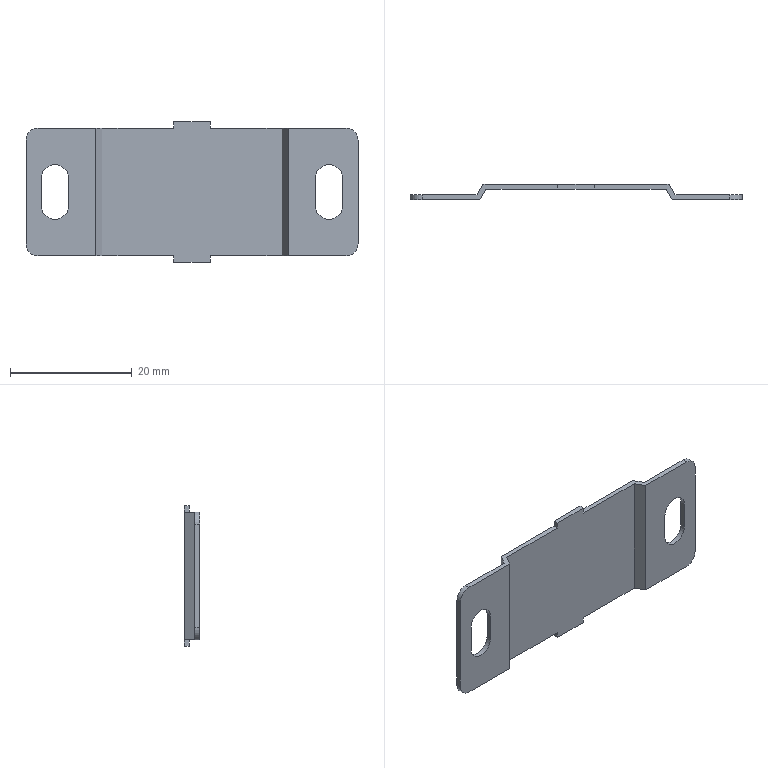Part | STEP file | Second C-100-B-2 Bracket Part | 1 solid | 34 faces | box 54.5 x 2.5 x 23 mm | volume 897.584 mm3 | plane 26 | cylinder 8 | commonest cylinder face diameters 4 x4 4.5 x4
STEP:
#1=CARTESIAN_POINT('',(3.,2.5,-11.5));
#2=VERTEX_POINT('',#1);
#3=CARTESIAN_POINT('',(3.,2.5,-10.5));
#4=VERTEX_POINT('',#3);
#5=CARTESIAN_POINT('',(3.,2.5,10.5));
#6=DIRECTION('',(0.,0.,1.));
#7=VECTOR('',#6,1000.);
#8=LINE('',#5,#7);
#9=EDGE_CURVE('',#2,#4,#8,.T.);
#10=ORIENTED_EDGE('',*,*,#9,.F.);
#11=CARTESIAN_POINT('',(-3.,2.5,-11.5));
#12=VERTEX_POINT('',#11);
#13=CARTESIAN_POINT('',(-15.269,2.5,-11.5));
#14=DIRECTION('',(1.,0.,0.));
#15=VECTOR('',#14,1000.);
#16=LINE('',#13,#15);
#17=EDGE_CURVE('',#12,#2,#16,.T.);
#18=ORIENTED_EDGE('',*,*,#17,.F.);
#19=CARTESIAN_POINT('',(-3.,2.5,-10.5));
#20=VERTEX_POINT('',#19);
#21=CARTESIAN_POINT('',(-3.,2.5,10.5));
#22=DIRECTION('',(0.,0.,-1.));
#23=VECTOR('',#22,1000.);
#24=LINE('',#21,#23);
#25=EDGE_CURVE('',#20,#12,#24,.T.);
#26=ORIENTED_EDGE('',*,*,#25,.F.);
#27=CARTESIAN_POINT('',(-15.269,2.5,-10.5));
#28=VERTEX_POINT('',#27);
#29=CARTESIAN_POINT('',(-15.269,2.5,-10.5));
#30=DIRECTION('',(1.,0.,0.));
#31=VECTOR('',#30,1000.);
#32=LINE('',#29,#31);
#33=EDGE_CURVE('',#28,#20,#32,.T.);
#34=ORIENTED_EDGE('',*,*,#33,.F.);
#35=CARTESIAN_POINT('',(-15.269,2.5,10.5));
#36=VERTEX_POINT('',#35);
#37=CARTESIAN_POINT('',(-15.269,2.5,10.5));
#38=DIRECTION('',(0.,0.,-1.));
#39=VECTOR('',#38,1000.);
#40=LINE('',#37,#39);
#41=EDGE_CURVE('',#36,#28,#40,.T.);
#42=ORIENTED_EDGE('',*,*,#41,.F.);
#43=CARTESIAN_POINT('',(-3.,2.5,10.5));
#44=VERTEX_POINT('',#43);
#45=CARTESIAN_POINT('',(-15.269,2.5,10.5));
#46=DIRECTION('',(-1.,0.,0.));
#47=VECTOR('',#46,1000.);
#48=LINE('',#45,#47);
#49=EDGE_CURVE('',#44,#36,#48,.T.);
#50=ORIENTED_EDGE('',*,*,#49,.F.);
#51=CARTESIAN_POINT('',(-3.,2.5,11.5));
#52=VERTEX_POINT('',#51);
#53=CARTESIAN_POINT('',(-3.,2.5,10.5));
#54=DIRECTION('',(0.,0.,-1.));
#55=VECTOR('',#54,1000.);
#56=LINE('',#53,#55);
#57=EDGE_CURVE('',#52,#44,#56,.T.);
#58=ORIENTED_EDGE('',*,*,#57,.F.);
#59=CARTESIAN_POINT('',(3.,2.5,11.5));
#60=VERTEX_POINT('',#59);
#61=CARTESIAN_POINT('',(-15.269,2.5,11.5));
#62=DIRECTION('',(-1.,0.,0.));
#63=VECTOR('',#62,1000.);
#64=LINE('',#61,#63);
#65=EDGE_CURVE('',#60,#52,#64,.T.);
#66=ORIENTED_EDGE('',*,*,#65,.F.);
#67=CARTESIAN_POINT('',(3.,2.5,10.5));
#68=VERTEX_POINT('',#67);
#69=CARTESIAN_POINT('',(3.,2.5,10.5));
#70=DIRECTION('',(0.,0.,1.));
#71=VECTOR('',#70,1000.);
#72=LINE('',#69,#71);
#73=EDGE_CURVE('',#68,#60,#72,.T.);
#74=ORIENTED_EDGE('',*,*,#73,.F.);
#75=CARTESIAN_POINT('',(15.269,2.5,10.5));
#76=VERTEX_POINT('',#75);
#77=CARTESIAN_POINT('',(-15.269,2.5,10.5));
#78=DIRECTION('',(-1.,0.,0.));
#79=VECTOR('',#78,1000.);
#80=LINE('',#77,#79);
#81=EDGE_CURVE('',#76,#68,#80,.T.);
#82=ORIENTED_EDGE('',*,*,#81,.F.);
#83=CARTESIAN_POINT('',(15.269,2.5,-10.5));
#84=VERTEX_POINT('',#83);
#85=CARTESIAN_POINT('',(15.269,2.5,10.5));
#86=DIRECTION('',(0.,0.,1.));
#87=VECTOR('',#86,1000.);
#88=LINE('',#85,#87);
#89=EDGE_CURVE('',#84,#76,#88,.T.);
#90=ORIENTED_EDGE('',*,*,#89,.F.);
#91=CARTESIAN_POINT('',(-15.269,2.5,-10.5));
#92=DIRECTION('',(1.,0.,0.));
#93=VECTOR('',#92,1000.);
#94=LINE('',#91,#93);
#95=EDGE_CURVE('',#4,#84,#94,.T.);
#96=ORIENTED_EDGE('',*,*,#95,.F.);
#97=EDGE_LOOP('',(#10,#18,#26,#34,#42,#50,#58,#66,#74,#82,#90,#96));
#98=FACE_OUTER_BOUND('',#97,.T.);
#99=CARTESIAN_POINT('',(-15.269,2.5,10.5));
#100=DIRECTION('',(0.,-1.,0.));
#101=DIRECTION('',(1.,0.,0.));
#102=AXIS2_PLACEMENT_3D('',#99,#100,#101);
#103=PLANE('',#102);
#104=ADVANCED_FACE('',(#98),#103,.F.);
#105=CARTESIAN_POINT('',(3.,1.7,-10.5));
#106=VERTEX_POINT('',#105);
#107=CARTESIAN_POINT('',(3.,2.5,-10.5));
#108=DIRECTION('',(0.,-1.,0.));
#109=VECTOR('',#108,1000.);
#110=LINE('',#107,#109);
#111=EDGE_CURVE('',#4,#106,#110,.T.);
#112=ORIENTED_EDGE('',*,*,#111,.F.);
#113=ORIENTED_EDGE('',*,*,#95,.T.);
#114=CARTESIAN_POINT('',(16.25,0.8,-10.5));
#115=VERTEX_POINT('',#114);
#116=CARTESIAN_POINT('',(16.25,0.8,-10.5));
#117=DIRECTION('',(-0.5,0.866,0.));
#118=VECTOR('',#117,1000.);
#119=LINE('',#116,#118);
#120=EDGE_CURVE('',#115,#84,#119,.T.);
#121=ORIENTED_EDGE('',*,*,#120,.F.);
#122=CARTESIAN_POINT('',(25.25,0.8,-10.5));
#123=VERTEX_POINT('',#122);
#124=CARTESIAN_POINT('',(-27.25,0.8,-10.5));
#125=DIRECTION('',(-1.,0.,0.));
#126=VECTOR('',#125,1000.);
#127=LINE('',#124,#126);
#128=EDGE_CURVE('',#123,#115,#127,.T.);
#129=ORIENTED_EDGE('',*,*,#128,.F.);
#130=CARTESIAN_POINT('',(25.25,0.,-10.5));
#131=VERTEX_POINT('',#130);
#132=CARTESIAN_POINT('',(25.25,0.,-10.5));
#133=DIRECTION('',(0.,1.,0.));
#134=VECTOR('',#133,1000.);
#135=LINE('',#132,#134);
#136=EDGE_CURVE('',#131,#123,#135,.T.);
#137=ORIENTED_EDGE('',*,*,#136,.F.);
#138=CARTESIAN_POINT('',(15.788,0.,-10.5));
#139=VERTEX_POINT('',#138);
#140=CARTESIAN_POINT('',(-27.25,0.,-10.5));
#141=DIRECTION('',(1.,0.,0.));
#142=VECTOR('',#141,1000.);
#143=LINE('',#140,#142);
#144=EDGE_CURVE('',#139,#131,#143,.T.);
#145=ORIENTED_EDGE('',*,*,#144,.F.);
#146=CARTESIAN_POINT('',(14.807,1.7,-10.5));
#147=VERTEX_POINT('',#146);
#148=CARTESIAN_POINT('',(14.807,1.7,-10.5));
#149=DIRECTION('',(0.5,-0.866,0.));
#150=VECTOR('',#149,1000.);
#151=LINE('',#148,#150);
#152=EDGE_CURVE('',#147,#139,#151,.T.);
#153=ORIENTED_EDGE('',*,*,#152,.F.);
#154=CARTESIAN_POINT('',(-27.25,1.7,-10.5));
#155=DIRECTION('',(1.,0.,0.));
#156=VECTOR('',#155,1000.);
#157=LINE('',#154,#156);
#158=EDGE_CURVE('',#106,#147,#157,.T.);
#159=ORIENTED_EDGE('',*,*,#158,.F.);
#160=EDGE_LOOP('',(#112,#113,#121,#129,#137,#145,#153,#159));
#161=FACE_OUTER_BOUND('',#160,.T.);
#162=CARTESIAN_POINT('',(-27.25,2.5,-10.5));
#163=DIRECTION('',(0.,0.,1.));
#164=DIRECTION('',(1.,0.,0.));
#165=AXIS2_PLACEMENT_3D('',#162,#163,#164);
#166=PLANE('',#165);
#167=ADVANCED_FACE('',(#161),#166,.F.);
#168=CARTESIAN_POINT('',(3.,1.7,-11.5));
#169=VERTEX_POINT('',#168);
#170=CARTESIAN_POINT('',(3.,1.7,-11.5));
#171=DIRECTION('',(0.,1.,0.));
#172=VECTOR('',#171,1000.);
#173=LINE('',#170,#172);
#174=EDGE_CURVE('',#169,#2,#173,.T.);
#175=ORIENTED_EDGE('',*,*,#174,.T.);
#176=ORIENTED_EDGE('',*,*,#9,.T.);
#177=ORIENTED_EDGE('',*,*,#111,.T.);
#178=CARTESIAN_POINT('',(3.,1.7,-11.5));
#179=DIRECTION('',(0.,0.,-1.));
#180=VECTOR('',#179,1000.);
#181=LINE('',#178,#180);
#182=EDGE_CURVE('',#106,#169,#181,.T.);
#183=ORIENTED_EDGE('',*,*,#182,.T.);
#184=EDGE_LOOP('',(#175,#176,#177,#183));
#185=FACE_OUTER_BOUND('',#184,.T.);
#186=CARTESIAN_POINT('',(3.,1.7,-11.5));
#187=DIRECTION('',(1.,0.,0.));
#188=DIRECTION('',(0.,1.,0.));
#189=AXIS2_PLACEMENT_3D('',#186,#187,#188);
#190=PLANE('',#189);
#191=ADVANCED_FACE('',(#185),#190,.T.);
#192=CARTESIAN_POINT('',(-3.,1.7,-11.5));
#193=VERTEX_POINT('',#192);
#194=CARTESIAN_POINT('',(-3.,1.7,-11.5));
#195=DIRECTION('',(-1.,0.,0.));
#196=VECTOR('',#195,1000.);
#197=LINE('',#194,#196);
#198=EDGE_CURVE('',#169,#193,#197,.T.);
#199=ORIENTED_EDGE('',*,*,#198,.T.);
#200=CARTESIAN_POINT('',(-3.,1.7,-11.5));
#201=DIRECTION('',(0.,1.,0.));
#202=VECTOR('',#201,1000.);
#203=LINE('',#200,#202);
#204=EDGE_CURVE('',#193,#12,#203,.T.);
#205=ORIENTED_EDGE('',*,*,#204,.T.);
#206=ORIENTED_EDGE('',*,*,#17,.T.);
#207=ORIENTED_EDGE('',*,*,#174,.F.);
#208=EDGE_LOOP('',(#199,#205,#206,#207));
#209=FACE_OUTER_BOUND('',#208,.T.);
#210=CARTESIAN_POINT('',(-3.,1.7,-11.5));
#211=DIRECTION('',(0.,0.,-1.));
#212=DIRECTION('',(-1.,0.,0.));
#213=AXIS2_PLACEMENT_3D('',#210,#211,#212);
#214=PLANE('',#213);
#215=ADVANCED_FACE('',(#209),#214,.T.);
#216=ORIENTED_EDGE('',*,*,#204,.F.);
#217=CARTESIAN_POINT('',(-3.,1.7,-10.5));
#218=VERTEX_POINT('',#217);
#219=CARTESIAN_POINT('',(-3.,1.7,11.5));
#220=DIRECTION('',(0.,0.,1.));
#221=VECTOR('',#220,1000.);
#222=LINE('',#219,#221);
#223=EDGE_CURVE('',#193,#218,#222,.T.);
#224=ORIENTED_EDGE('',*,*,#223,.T.);
#225=CARTESIAN_POINT('',(-3.,1.7,-10.5));
#226=DIRECTION('',(0.,1.,0.));
#227=VECTOR('',#226,1000.);
#228=LINE('',#225,#227);
#229=EDGE_CURVE('',#218,#20,#228,.T.);
#230=ORIENTED_EDGE('',*,*,#229,.T.);
#231=ORIENTED_EDGE('',*,*,#25,.T.);
#232=EDGE_LOOP('',(#216,#224,#230,#231));
#233=FACE_OUTER_BOUND('',#232,.T.);
#234=CARTESIAN_POINT('',(-3.,1.7,11.5));
#235=DIRECTION('',(-1.,0.,0.));
#236=DIRECTION('',(0.,0.,1.));
#237=AXIS2_PLACEMENT_3D('',#234,#235,#236);
#238=PLANE('',#237);
#239=ADVANCED_FACE('',(#233),#238,.T.);
#240=ORIENTED_EDGE('',*,*,#229,.F.);
#241=CARTESIAN_POINT('',(-14.807,1.7,-10.5));
#242=VERTEX_POINT('',#241);
#243=CARTESIAN_POINT('',(-27.25,1.7,-10.5));
#244=DIRECTION('',(1.,0.,0.));
#245=VECTOR('',#244,1000.);
#246=LINE('',#243,#245);
#247=EDGE_CURVE('',#242,#218,#246,.T.);
#248=ORIENTED_EDGE('',*,*,#247,.F.);
#249=CARTESIAN_POINT('',(-15.788,0.,-10.5));
#250=VERTEX_POINT('',#249);
#251=CARTESIAN_POINT('',(-15.788,0.,-10.5));
#252=DIRECTION('',(0.5,0.866,0.));
#253=VECTOR('',#252,1000.);
#254=LINE('',#251,#253);
#255=EDGE_CURVE('',#250,#242,#254,.T.);
#256=ORIENTED_EDGE('',*,*,#255,.F.);
#257=CARTESIAN_POINT('',(-25.25,0.,-10.5));
#258=VERTEX_POINT('',#257);
#259=CARTESIAN_POINT('',(-27.25,0.,-10.5));
#260=DIRECTION('',(1.,0.,0.));
#261=VECTOR('',#260,1000.);
#262=LINE('',#259,#261);
#263=EDGE_CURVE('',#258,#250,#262,.T.);
#264=ORIENTED_EDGE('',*,*,#263,.F.);
#265=CARTESIAN_POINT('',(-25.25,0.8,-10.5));
#266=VERTEX_POINT('',#265);
#267=CARTESIAN_POINT('',(-25.25,0.8,-10.5));
#268=DIRECTION('',(0.,-1.,0.));
#269=VECTOR('',#268,1000.);
#270=LINE('',#267,#269);
#271=EDGE_CURVE('',#266,#258,#270,.T.);
#272=ORIENTED_EDGE('',*,*,#271,.F.);
#273=CARTESIAN_POINT('',(-16.25,0.8,-10.5));
#274=VERTEX_POINT('',#273);
#275=CARTESIAN_POINT('',(-27.25,0.8,-10.5));
#276=DIRECTION('',(-1.,0.,0.));
#277=VECTOR('',#276,1000.);
#278=LINE('',#275,#277);
#279=EDGE_CURVE('',#274,#266,#278,.T.);
#280=ORIENTED_EDGE('',*,*,#279,.F.);
#281=CARTESIAN_POINT('',(-15.269,2.5,-10.5));
#282=DIRECTION('',(-0.5,-0.866,0.));
#283=VECTOR('',#282,1000.);
#284=LINE('',#281,#283);
#285=EDGE_CURVE('',#28,#274,#284,.T.);
#286=ORIENTED_EDGE('',*,*,#285,.F.);
#287=ORIENTED_EDGE('',*,*,#33,.T.);
#288=EDGE_LOOP('',(#240,#248,#256,#264,#272,#280,#286,#287));
#289=FACE_OUTER_BOUND('',#288,.T.);
#290=CARTESIAN_POINT('',(-27.25,2.5,-10.5));
#291=DIRECTION('',(0.,0.,1.));
#292=DIRECTION('',(1.,0.,0.));
#293=AXIS2_PLACEMENT_3D('',#290,#291,#292);
#294=PLANE('',#293);
#295=ADVANCED_FACE('',(#289),#294,.F.);
#296=ORIENTED_EDGE('',*,*,#285,.T.);
#297=CARTESIAN_POINT('',(-16.25,0.8,10.5));
#298=VERTEX_POINT('',#297);
#299=CARTESIAN_POINT('',(-16.25,0.8,10.5));
#300=DIRECTION('',(0.,0.,-1.));
#301=VECTOR('',#300,1000.);
#302=LINE('',#299,#301);
#303=EDGE_CURVE('',#298,#274,#302,.T.);
#304=ORIENTED_EDGE('',*,*,#303,.F.);
#305=CARTESIAN_POINT('',(-16.25,0.8,10.5));
#306=DIRECTION('',(-0.5,-0.866,0.));
#307=VECTOR('',#306,1000.);
#308=LINE('',#305,#307);
#309=EDGE_CURVE('',#36,#298,#308,.T.);
#310=ORIENTED_EDGE('',*,*,#309,.F.);
#311=ORIENTED_EDGE('',*,*,#41,.T.);
#312=EDGE_LOOP('',(#296,#304,#310,#311));
#313=FACE_OUTER_BOUND('',#312,.T.);
#314=CARTESIAN_POINT('',(-16.25,0.8,10.5));
#315=DIRECTION('',(0.866,-0.5,0.));
#316=DIRECTION('',(0.5,0.866,0.));
#317=AXIS2_PLACEMENT_3D('',#314,#315,#316);
#318=PLANE('',#317);
#319=ADVANCED_FACE('',(#313),#318,.F.);
#320=CARTESIAN_POINT('',(-15.788,0.,10.5));
#321=VERTEX_POINT('',#320);
#322=CARTESIAN_POINT('',(-14.807,1.7,10.5));
#323=VERTEX_POINT('',#322);
#324=CARTESIAN_POINT('',(-15.788,0.,10.5));
#325=DIRECTION('',(0.5,0.866,0.));
#326=VECTOR('',#325,1000.);
#327=LINE('',#324,#326);
#328=EDGE_CURVE('',#321,#323,#327,.T.);
#329=ORIENTED_EDGE('',*,*,#328,.T.);
#330=CARTESIAN_POINT('',(-3.,1.7,10.5));
#331=VERTEX_POINT('',#330);
#332=CARTESIAN_POINT('',(-27.25,1.7,10.5));
#333=DIRECTION('',(1.,0.,0.));
#334=VECTOR('',#333,1000.);
#335=LINE('',#332,#334);
#336=EDGE_CURVE('',#323,#331,#335,.T.);
#337=ORIENTED_EDGE('',*,*,#336,.T.);
#338=CARTESIAN_POINT('',(-3.,2.5,10.5));
#339=DIRECTION('',(0.,1.,0.));
#340=VECTOR('',#339,1000.);
#341=LINE('',#338,#340);
#342=EDGE_CURVE('',#331,#44,#341,.T.);
#343=ORIENTED_EDGE('',*,*,#342,.T.);
#344=ORIENTED_EDGE('',*,*,#49,.T.);
#345=ORIENTED_EDGE('',*,*,#309,.T.);
#346=CARTESIAN_POINT('',(-25.25,0.8,10.5));
#347=VERTEX_POINT('',#346);
#348=CARTESIAN_POINT('',(-27.25,0.8,10.5));
#349=DIRECTION('',(-1.,0.,0.));
#350=VECTOR('',#349,1000.);
#351=LINE('',#348,#350);
#352=EDGE_CURVE('',#298,#347,#351,.T.);
#353=ORIENTED_EDGE('',*,*,#352,.T.);
#354=CARTESIAN_POINT('',(-25.25,0.,10.5));
#355=VERTEX_POINT('',#354);
#356=CARTESIAN_POINT('',(-25.25,2.5,10.5));
#357=DIRECTION('',(0.,1.,0.));
#358=VECTOR('',#357,1000.);
#359=LINE('',#356,#358);
#360=EDGE_CURVE('',#355,#347,#359,.T.);
#361=ORIENTED_EDGE('',*,*,#360,.F.);
#362=CARTESIAN_POINT('',(-27.25,0.,10.5));
#363=DIRECTION('',(1.,0.,0.));
#364=VECTOR('',#363,1000.);
#365=LINE('',#362,#364);
#366=EDGE_CURVE('',#355,#321,#365,.T.);
#367=ORIENTED_EDGE('',*,*,#366,.T.);
#368=EDGE_LOOP('',(#329,#337,#343,#344,#345,#353,#361,#367));
#369=FACE_OUTER_BOUND('',#368,.T.);
#370=CARTESIAN_POINT('',(-27.25,2.5,10.5));
#371=DIRECTION('',(0.,0.,1.));
#372=DIRECTION('',(1.,0.,0.));
#373=AXIS2_PLACEMENT_3D('',#370,#371,#372);
#374=PLANE('',#373);
#375=ADVANCED_FACE('',(#369),#374,.T.);
#376=CARTESIAN_POINT('',(-3.,1.7,11.5));
#377=VERTEX_POINT('',#376);
#378=CARTESIAN_POINT('',(-3.,1.7,11.5));
#379=DIRECTION('',(0.,0.,1.));
#380=VECTOR('',#379,1000.);
#381=LINE('',#378,#380);
#382=EDGE_CURVE('',#331,#377,#381,.T.);
#383=ORIENTED_EDGE('',*,*,#382,.T.);
#384=CARTESIAN_POINT('',(-3.,1.7,11.5));
#385=DIRECTION('',(0.,1.,0.));
#386=VECTOR('',#385,1000.);
#387=LINE('',#384,#386);
#388=EDGE_CURVE('',#377,#52,#387,.T.);
#389=ORIENTED_EDGE('',*,*,#388,.T.);
#390=ORIENTED_EDGE('',*,*,#57,.T.);
#391=ORIENTED_EDGE('',*,*,#342,.F.);
#392=EDGE_LOOP('',(#383,#389,#390,#391));
#393=FACE_OUTER_BOUND('',#392,.T.);
#394=CARTESIAN_POINT('',(-3.,1.7,11.5));
#395=DIRECTION('',(-1.,0.,0.));
#396=DIRECTION('',(0.,0.,1.));
#397=AXIS2_PLACEMENT_3D('',#394,#395,#396);
#398=PLANE('',#397);
#399=ADVANCED_FACE('',(#393),#398,.T.);
#400=CARTESIAN_POINT('',(3.,1.7,11.5));
#401=VERTEX_POINT('',#400);
#402=CARTESIAN_POINT('',(3.,1.7,11.5));
#403=DIRECTION('',(1.,0.,0.));
#404=VECTOR('',#403,1000.);
#405=LINE('',#402,#404);
#406=EDGE_CURVE('',#377,#401,#405,.T.);
#407=ORIENTED_EDGE('',*,*,#406,.T.);
#408=CARTESIAN_POINT('',(3.,1.7,11.5));
#409=DIRECTION('',(0.,1.,0.));
#410=VECTOR('',#409,1000.);
#411=LINE('',#408,#410);
#412=EDGE_CURVE('',#401,#60,#411,.T.);
#413=ORIENTED_EDGE('',*,*,#412,.T.);
#414=ORIENTED_EDGE('',*,*,#65,.T.);
#415=ORIENTED_EDGE('',*,*,#388,.F.);
#416=EDGE_LOOP('',(#407,#413,#414,#415));
#417=FACE_OUTER_BOUND('',#416,.T.);
#418=CARTESIAN_POINT('',(3.,1.7,11.5));
#419=DIRECTION('',(0.,0.,1.));
#420=DIRECTION('',(1.,0.,0.));
#421=AXIS2_PLACEMENT_3D('',#418,#419,#420);
#422=PLANE('',#421);
#423=ADVANCED_FACE('',(#417),#422,.T.);
#424=ORIENTED_EDGE('',*,*,#73,.T.);
#425=ORIENTED_EDGE('',*,*,#412,.F.);
#426=CARTESIAN_POINT('',(3.,1.7,10.5));
#427=VERTEX_POINT('',#426);
#428=CARTESIAN_POINT('',(3.,1.7,-11.5));
#429=DIRECTION('',(0.,0.,-1.));
#430=VECTOR('',#429,1000.);
#431=LINE('',#428,#430);
#432=EDGE_CURVE('',#401,#427,#431,.T.);
#433=ORIENTED_EDGE('',*,*,#432,.T.);
#434=CARTESIAN_POINT('',(3.,1.7,10.5));
#435=DIRECTION('',(0.,1.,0.));
#436=VECTOR('',#435,1000.);
#437=LINE('',#434,#436);
#438=EDGE_CURVE('',#427,#68,#437,.T.);
#439=ORIENTED_EDGE('',*,*,#438,.T.);
#440=EDGE_LOOP('',(#424,#425,#433,#439));
#441=FACE_OUTER_BOUND('',#440,.T.);
#442=CARTESIAN_POINT('',(3.,1.7,-11.5));
#443=DIRECTION('',(1.,0.,0.));
#444=DIRECTION('',(0.,1.,0.));
#445=AXIS2_PLACEMENT_3D('',#442,#443,#444);
#446=PLANE('',#445);
#447=ADVANCED_FACE('',(#441),#446,.T.);
#448=CARTESIAN_POINT('',(16.25,0.8,10.5));
#449=VERTEX_POINT('',#448);
#450=CARTESIAN_POINT('',(16.25,0.8,10.5));
#451=DIRECTION('',(-0.5,0.866,0.));
#452=VECTOR('',#451,1000.);
#453=LINE('',#450,#452);
#454=EDGE_CURVE('',#449,#76,#453,.T.);
#455=ORIENTED_EDGE('',*,*,#454,.T.);
#456=ORIENTED_EDGE('',*,*,#81,.T.);
#457=ORIENTED_EDGE('',*,*,#438,.F.);
#458=CARTESIAN_POINT('',(14.807,1.7,10.5));
#459=VERTEX_POINT('',#458);
#460=CARTESIAN_POINT('',(-27.25,1.7,10.5));
#461=DIRECTION('',(1.,0.,0.));
#462=VECTOR('',#461,1000.);
#463=LINE('',#460,#462);
#464=EDGE_CURVE('',#427,#459,#463,.T.);
#465=ORIENTED_EDGE('',*,*,#464,.T.);
#466=CARTESIAN_POINT('',(15.788,0.,10.5));
#467=VERTEX_POINT('',#466);
#468=CARTESIAN_POINT('',(14.807,1.7,10.5));
#469=DIRECTION('',(0.5,-0.866,0.));
#470=VECTOR('',#469,1000.);
#471=LINE('',#468,#470);
#472=EDGE_CURVE('',#459,#467,#471,.T.);
#473=ORIENTED_EDGE('',*,*,#472,.T.);
#474=CARTESIAN_POINT('',(25.25,0.,10.5));
#475=VERTEX_POINT('',#474);
#476=CARTESIAN_POINT('',(-27.25,0.,10.5));
#477=DIRECTION('',(1.,0.,0.));
#478=VECTOR('',#477,1000.);
#479=LINE('',#476,#478);
#480=EDGE_CURVE('',#467,#475,#479,.T.);
#481=ORIENTED_EDGE('',*,*,#480,.T.);
#482=CARTESIAN_POINT('',(25.25,0.8,10.5));
#483=VERTEX_POINT('',#482);
#484=CARTESIAN_POINT('',(25.25,2.5,10.5));
#485=DIRECTION('',(0.,-1.,0.));
#486=VECTOR('',#485,1000.);
#487=LINE('',#484,#486);
#488=EDGE_CURVE('',#483,#475,#487,.T.);
#489=ORIENTED_EDGE('',*,*,#488,.F.);
#490=CARTESIAN_POINT('',(-27.25,0.8,10.5));
#491=DIRECTION('',(-1.,0.,0.));
#492=VECTOR('',#491,1000.);
#493=LINE('',#490,#492);
#494=EDGE_CURVE('',#483,#449,#493,.T.);
#495=ORIENTED_EDGE('',*,*,#494,.T.);
#496=EDGE_LOOP('',(#455,#456,#457,#465,#473,#481,#489,#495));
#497=FACE_OUTER_BOUND('',#496,.T.);
#498=CARTESIAN_POINT('',(-27.25,2.5,10.5));
#499=DIRECTION('',(0.,0.,1.));
#500=DIRECTION('',(1.,0.,0.));
#501=AXIS2_PLACEMENT_3D('',#498,#499,#500);
#502=PLANE('',#501);
#503=ADVANCED_FACE('',(#497),#502,.T.);
#504=ORIENTED_EDGE('',*,*,#120,.T.);
#505=ORIENTED_EDGE('',*,*,#89,.T.);
#506=ORIENTED_EDGE('',*,*,#454,.F.);
#507=CARTESIAN_POINT('',(16.25,0.8,10.5));
#508=DIRECTION('',(0.,0.,1.));
#509=VECTOR('',#508,1000.);
#510=LINE('',#507,#509);
#511=EDGE_CURVE('',#115,#449,#510,.T.);
#512=ORIENTED_EDGE('',*,*,#511,.F.);
#513=EDGE_LOOP('',(#504,#505,#506,#512));
#514=FACE_OUTER_BOUND('',#513,.T.);
#515=CARTESIAN_POINT('',(16.25,0.8,10.5));
#516=DIRECTION('',(-0.866,-0.5,0.));
#517=DIRECTION('',(0.5,-0.866,0.));
#518=AXIS2_PLACEMENT_3D('',#515,#516,#517);
#519=PLANE('',#518);
#520=ADVANCED_FACE('',(#514),#519,.F.);
#521=ORIENTED_EDGE('',*,*,#432,.F.);
#522=ORIENTED_EDGE('',*,*,#406,.F.);
#523=ORIENTED_EDGE('',*,*,#382,.F.);
#524=ORIENTED_EDGE('',*,*,#336,.F.);
#525=CARTESIAN_POINT('',(-14.807,1.7,10.5));
#526=DIRECTION('',(0.,0.,1.));
#527=VECTOR('',#526,1000.);
#528=LINE('',#525,#527);
#529=EDGE_CURVE('',#242,#323,#528,.T.);
#530=ORIENTED_EDGE('',*,*,#529,.F.);
#531=ORIENTED_EDGE('',*,*,#247,.T.);
#532=ORIENTED_EDGE('',*,*,#223,.F.);
#533=ORIENTED_EDGE('',*,*,#198,.F.);
#534=ORIENTED_EDGE('',*,*,#182,.F.);
#535=ORIENTED_EDGE('',*,*,#158,.T.);
#536=CARTESIAN_POINT('',(14.807,1.7,10.5));
#537=DIRECTION('',(0.,0.,-1.));
#538=VECTOR('',#537,1000.);
#539=LINE('',#536,#538);
#540=EDGE_CURVE('',#459,#147,#539,.T.);
#541=ORIENTED_EDGE('',*,*,#540,.F.);
#542=ORIENTED_EDGE('',*,*,#464,.F.);
#543=EDGE_LOOP('',(#521,#522,#523,#524,#530,#531,#532,#533,#534,#535,#541,#542));
#544=FACE_OUTER_BOUND('',#543,.T.);
#545=CARTESIAN_POINT('',(-14.807,1.7,10.5));
#546=DIRECTION('',(0.,1.,0.));
#547=DIRECTION('',(-1.,0.,0.));
#548=AXIS2_PLACEMENT_3D('',#545,#546,#547);
#549=PLANE('',#548);
#550=ADVANCED_FACE('',(#544),#549,.F.);
#551=CARTESIAN_POINT('',(27.25,0.8,-8.5));
#552=VERTEX_POINT('',#551);
#553=CARTESIAN_POINT('',(25.25,0.8,-8.5));
#554=DIRECTION('',(0.,-1.,0.));
#555=DIRECTION('',(-1.,0.,0.));
#556=AXIS2_PLACEMENT_3D('',#553,#554,#555);
#557=CIRCLE('',#556,2.);
#558=EDGE_CURVE('',#123,#552,#557,.T.);
#559=ORIENTED_EDGE('',*,*,#558,.F.);
#560=ORIENTED_EDGE('',*,*,#128,.T.);
#561=ORIENTED_EDGE('',*,*,#511,.T.);
#562=ORIENTED_EDGE('',*,*,#494,.F.);
#563=CARTESIAN_POINT('',(27.25,0.8,8.5));
#564=VERTEX_POINT('',#563);
#565=CARTESIAN_POINT('',(25.25,0.8,8.5));
#566=DIRECTION('',(0.,-1.,0.));
#567=DIRECTION('',(1.,0.,0.));
#568=AXIS2_PLACEMENT_3D('',#565,#566,#567);
#569=CIRCLE('',#568,2.);
#570=EDGE_CURVE('',#564,#483,#569,.T.);
#571=ORIENTED_EDGE('',*,*,#570,.F.);
#572=CARTESIAN_POINT('',(27.25,0.8,10.5));
#573=DIRECTION('',(0.,0.,1.));
#574=VECTOR('',#573,1000.);
#575=LINE('',#572,#574);
#576=EDGE_CURVE('',#552,#564,#575,.T.);
#577=ORIENTED_EDGE('',*,*,#576,.F.);
#578=EDGE_LOOP('',(#559,#560,#561,#562,#571,#577));
#579=FACE_OUTER_BOUND('',#578,.T.);
#580=CARTESIAN_POINT('',(24.75,0.8,-2.25));
#581=VERTEX_POINT('',#580);
#582=CARTESIAN_POINT('',(20.25,0.8,-2.25));
#583=VERTEX_POINT('',#582);
#584=CARTESIAN_POINT('',(22.5,0.8,-2.25));
#585=DIRECTION('',(0.,1.,0.));
#586=DIRECTION('',(-1.,0.,0.));
#587=AXIS2_PLACEMENT_3D('',#584,#585,#586);
#588=CIRCLE('',#587,2.25);
#589=EDGE_CURVE('',#581,#583,#588,.T.);
#590=ORIENTED_EDGE('',*,*,#589,.F.);
#591=CARTESIAN_POINT('',(24.75,0.8,2.25));
#592=VERTEX_POINT('',#591);
#593=CARTESIAN_POINT('',(24.75,0.8,10.5));
#594=DIRECTION('',(0.,0.,-1.));
#595=VECTOR('',#594,1000.);
#596=LINE('',#593,#595);
#597=EDGE_CURVE('',#592,#581,#596,.T.);
#598=ORIENTED_EDGE('',*,*,#597,.F.);
#599=CARTESIAN_POINT('',(20.25,0.8,2.25));
#600=VERTEX_POINT('',#599);
#601=CARTESIAN_POINT('',(22.5,0.8,2.25));
#602=DIRECTION('',(0.,1.,0.));
#603=DIRECTION('',(-1.,0.,0.));
#604=AXIS2_PLACEMENT_3D('',#601,#602,#603);
#605=CIRCLE('',#604,2.25);
#606=EDGE_CURVE('',#600,#592,#605,.T.);
#607=ORIENTED_EDGE('',*,*,#606,.F.);
#608=CARTESIAN_POINT('',(20.25,0.8,10.5));
#609=DIRECTION('',(0.,0.,1.));
#610=VECTOR('',#609,1000.);
#611=LINE('',#608,#610);
#612=EDGE_CURVE('',#583,#600,#611,.T.);
#613=ORIENTED_EDGE('',*,*,#612,.F.);
#614=EDGE_LOOP('',(#590,#598,#607,#613));
#615=FACE_BOUND('',#614,.T.);
#616=CARTESIAN_POINT('',(27.25,0.8,10.5));
#617=DIRECTION('',(0.,-1.,0.));
#618=DIRECTION('',(1.,0.,0.));
#619=AXIS2_PLACEMENT_3D('',#616,#617,#618);
#620=PLANE('',#619);
#621=ADVANCED_FACE('',(#579,#615),#620,.F.);
#622=CARTESIAN_POINT('',(27.25,0.,-8.5));
#623=VERTEX_POINT('',#622);
#624=CARTESIAN_POINT('',(25.25,0.,-8.5));
#625=DIRECTION('',(0.,1.,0.));
#626=DIRECTION('',(-1.,0.,0.));
#627=AXIS2_PLACEMENT_3D('',#624,#625,#626);
#628=CIRCLE('',#627,2.);
#629=EDGE_CURVE('',#623,#131,#628,.T.);
#630=ORIENTED_EDGE('',*,*,#629,.F.);
#631=CARTESIAN_POINT('',(27.25,0.,8.5));
#632=VERTEX_POINT('',#631);
#633=CARTESIAN_POINT('',(27.25,0.,10.5));
#634=DIRECTION('',(0.,0.,-1.));
#635=VECTOR('',#634,1000.);
#636=LINE('',#633,#635);
#637=EDGE_CURVE('',#632,#623,#636,.T.);
#638=ORIENTED_EDGE('',*,*,#637,.F.);
#639=CARTESIAN_POINT('',(25.25,0.,8.5));
#640=DIRECTION('',(0.,1.,0.));
#641=DIRECTION('',(1.,0.,0.));
#642=AXIS2_PLACEMENT_3D('',#639,#640,#641);
#643=CIRCLE('',#642,2.);
#644=EDGE_CURVE('',#475,#632,#643,.T.);
#645=ORIENTED_EDGE('',*,*,#644,.F.);
#646=ORIENTED_EDGE('',*,*,#480,.F.);
#647=CARTESIAN_POINT('',(15.788,0.,10.5));
#648=DIRECTION('',(0.,0.,1.));
#649=VECTOR('',#648,1000.);
#650=LINE('',#647,#649);
#651=EDGE_CURVE('',#139,#467,#650,.T.);
#652=ORIENTED_EDGE('',*,*,#651,.F.);
#653=ORIENTED_EDGE('',*,*,#144,.T.);
#654=EDGE_LOOP('',(#630,#638,#645,#646,#652,#653));
#655=FACE_OUTER_BOUND('',#654,.T.);
#656=CARTESIAN_POINT('',(20.25,0.,-2.25));
#657=VERTEX_POINT('',#656);
#658=CARTESIAN_POINT('',(24.75,0.,-2.25));
#659=VERTEX_POINT('',#658);
#660=CARTESIAN_POINT('',(22.5,0.,-2.25));
#661=DIRECTION('',(0.,-1.,0.));
#662=DIRECTION('',(-1.,0.,0.));
#663=AXIS2_PLACEMENT_3D('',#660,#661,#662);
#664=CIRCLE('',#663,2.25);
#665=EDGE_CURVE('',#657,#659,#664,.T.);
#666=ORIENTED_EDGE('',*,*,#665,.F.);
#667=CARTESIAN_POINT('',(20.25,0.,2.25));
#668=VERTEX_POINT('',#667);
#669=CARTESIAN_POINT('',(20.25,0.,10.5));
#670=DIRECTION('',(0.,0.,-1.));
#671=VECTOR('',#670,1000.);
#672=LINE('',#669,#671);
#673=EDGE_CURVE('',#668,#657,#672,.T.);
#674=ORIENTED_EDGE('',*,*,#673,.F.);
#675=CARTESIAN_POINT('',(24.75,0.,2.25));
#676=VERTEX_POINT('',#675);
#677=CARTESIAN_POINT('',(22.5,0.,2.25));
#678=DIRECTION('',(0.,-1.,0.));
#679=DIRECTION('',(-1.,0.,0.));
#680=AXIS2_PLACEMENT_3D('',#677,#678,#679);
#681=CIRCLE('',#680,2.25);
#682=EDGE_CURVE('',#676,#668,#681,.T.);
#683=ORIENTED_EDGE('',*,*,#682,.F.);
#684=CARTESIAN_POINT('',(24.75,0.,10.5));
#685=DIRECTION('',(0.,0.,1.));
#686=VECTOR('',#685,1000.);
#687=LINE('',#684,#686);
#688=EDGE_CURVE('',#659,#676,#687,.T.);
#689=ORIENTED_EDGE('',*,*,#688,.F.);
#690=EDGE_LOOP('',(#666,#674,#683,#689));
#691=FACE_BOUND('',#690,.T.);
#692=CARTESIAN_POINT('',(15.788,0.,10.5));
#693=DIRECTION('',(0.,1.,0.));
#694=DIRECTION('',(-1.,0.,0.));
#695=AXIS2_PLACEMENT_3D('',#692,#693,#694);
#696=PLANE('',#695);
#697=ADVANCED_FACE('',(#655,#691),#696,.F.);
#698=ORIENTED_EDGE('',*,*,#152,.T.);
#699=ORIENTED_EDGE('',*,*,#651,.T.);
#700=ORIENTED_EDGE('',*,*,#472,.F.);
#701=ORIENTED_EDGE('',*,*,#540,.T.);
#702=EDGE_LOOP('',(#698,#699,#700,#701));
#703=FACE_OUTER_BOUND('',#702,.T.);
#704=CARTESIAN_POINT('',(14.807,1.7,10.5));
#705=DIRECTION('',(0.866,0.5,0.));
#706=DIRECTION('',(-0.5,0.866,0.));
#707=AXIS2_PLACEMENT_3D('',#704,#705,#706);
#708=PLANE('',#707);
#709=ADVANCED_FACE('',(#703),#708,.F.);
#710=ORIENTED_EDGE('',*,*,#255,.T.);
#711=ORIENTED_EDGE('',*,*,#529,.T.);
#712=ORIENTED_EDGE('',*,*,#328,.F.);
#713=CARTESIAN_POINT('',(-15.788,0.,10.5));
#714=DIRECTION('',(0.,0.,1.));
#715=VECTOR('',#714,1000.);
#716=LINE('',#713,#715);
#717=EDGE_CURVE('',#250,#321,#716,.T.);
#718=ORIENTED_EDGE('',*,*,#717,.F.);
#719=EDGE_LOOP('',(#710,#711,#712,#718));
#720=FACE_OUTER_BOUND('',#719,.T.);
#721=CARTESIAN_POINT('',(-14.807,1.7,10.5));
#722=DIRECTION('',(-0.866,0.5,0.));
#723=DIRECTION('',(-0.5,-0.866,0.));
#724=AXIS2_PLACEMENT_3D('',#721,#722,#723);
#725=PLANE('',#724);
#726=ADVANCED_FACE('',(#720),#725,.F.);
#727=CARTESIAN_POINT('',(-27.25,0.,8.5));
#728=VERTEX_POINT('',#727);
#729=CARTESIAN_POINT('',(-25.25,0.,8.5));
#730=DIRECTION('',(0.,1.,0.));
#731=DIRECTION('',(0.,0.,1.));
#732=AXIS2_PLACEMENT_3D('',#729,#730,#731);
#733=CIRCLE('',#732,2.);
#734=EDGE_CURVE('',#728,#355,#733,.T.);
#735=ORIENTED_EDGE('',*,*,#734,.F.);
#736=CARTESIAN_POINT('',(-27.25,0.,-8.5));
#737=VERTEX_POINT('',#736);
#738=CARTESIAN_POINT('',(-27.25,0.,10.5));
#739=DIRECTION('',(0.,0.,1.));
#740=VECTOR('',#739,1000.);
#741=LINE('',#738,#740);
#742=EDGE_CURVE('',#737,#728,#741,.T.);
#743=ORIENTED_EDGE('',*,*,#742,.F.);
#744=CARTESIAN_POINT('',(-25.25,0.,-8.5));
#745=DIRECTION('',(0.,1.,0.));
#746=DIRECTION('',(0.,0.,-1.));
#747=AXIS2_PLACEMENT_3D('',#744,#745,#746);
#748=CIRCLE('',#747,2.);
#749=EDGE_CURVE('',#258,#737,#748,.T.);
#750=ORIENTED_EDGE('',*,*,#749,.F.);
#751=ORIENTED_EDGE('',*,*,#263,.T.);
#752=ORIENTED_EDGE('',*,*,#717,.T.);
#753=ORIENTED_EDGE('',*,*,#366,.F.);
#754=EDGE_LOOP('',(#735,#743,#750,#751,#752,#753));
#755=FACE_OUTER_BOUND('',#754,.T.);
#756=CARTESIAN_POINT('',(-20.25,0.,2.25));
#757=VERTEX_POINT('',#756);
#758=CARTESIAN_POINT('',(-24.75,0.,2.25));
#759=VERTEX_POINT('',#758);
#760=CARTESIAN_POINT('',(-22.5,0.,2.25));
#761=DIRECTION('',(0.,-1.,0.));
#762=DIRECTION('',(-1.,0.,0.));
#763=AXIS2_PLACEMENT_3D('',#760,#761,#762);
#764=CIRCLE('',#763,2.25);
#765=EDGE_CURVE('',#757,#759,#764,.T.);
#766=ORIENTED_EDGE('',*,*,#765,.F.);
#767=CARTESIAN_POINT('',(-20.25,0.,-2.25));
#768=VERTEX_POINT('',#767);
#769=CARTESIAN_POINT('',(-20.25,0.,10.5));
#770=DIRECTION('',(0.,0.,1.));
#771=VECTOR('',#770,1000.);
#772=LINE('',#769,#771);
#773=EDGE_CURVE('',#768,#757,#772,.T.);
#774=ORIENTED_EDGE('',*,*,#773,.F.);
#775=CARTESIAN_POINT('',(-24.75,0.,-2.25));
#776=VERTEX_POINT('',#775);
#777=CARTESIAN_POINT('',(-22.5,0.,-2.25));
#778=DIRECTION('',(0.,-1.,0.));
#779=DIRECTION('',(-1.,0.,0.));
#780=AXIS2_PLACEMENT_3D('',#777,#778,#779);
#781=CIRCLE('',#780,2.25);
#782=EDGE_CURVE('',#776,#768,#781,.T.);
#783=ORIENTED_EDGE('',*,*,#782,.F.);
#784=CARTESIAN_POINT('',(-24.75,0.,10.5));
#785=DIRECTION('',(0.,0.,-1.));
#786=VECTOR('',#785,1000.);
#787=LINE('',#784,#786);
#788=EDGE_CURVE('',#759,#776,#787,.T.);
#789=ORIENTED_EDGE('',*,*,#788,.F.);
#790=EDGE_LOOP('',(#766,#774,#783,#789));
#791=FACE_BOUND('',#790,.T.);
#792=CARTESIAN_POINT('',(-27.25,0.,10.5));
#793=DIRECTION('',(0.,1.,0.));
#794=DIRECTION('',(-1.,0.,0.));
#795=AXIS2_PLACEMENT_3D('',#792,#793,#794);
#796=PLANE('',#795);
#797=ADVANCED_FACE('',(#755,#791),#796,.F.);
#798=CARTESIAN_POINT('',(-27.25,0.8,8.5));
#799=VERTEX_POINT('',#798);
#800=CARTESIAN_POINT('',(-25.25,0.8,8.5));
#801=DIRECTION('',(0.,-1.,0.));
#802=DIRECTION('',(0.,0.,1.));
#803=AXIS2_PLACEMENT_3D('',#800,#801,#802);
#804=CIRCLE('',#803,2.);
#805=EDGE_CURVE('',#347,#799,#804,.T.);
#806=ORIENTED_EDGE('',*,*,#805,.F.);
#807=ORIENTED_EDGE('',*,*,#352,.F.);
#808=ORIENTED_EDGE('',*,*,#303,.T.);
#809=ORIENTED_EDGE('',*,*,#279,.T.);
#810=CARTESIAN_POINT('',(-27.25,0.8,-8.5));
#811=VERTEX_POINT('',#810);
#812=CARTESIAN_POINT('',(-25.25,0.8,-8.5));
#813=DIRECTION('',(0.,-1.,0.));
#814=DIRECTION('',(0.,0.,-1.));
#815=AXIS2_PLACEMENT_3D('',#812,#813,#814);
#816=CIRCLE('',#815,2.);
#817=EDGE_CURVE('',#811,#266,#816,.T.);
#818=ORIENTED_EDGE('',*,*,#817,.F.);
#819=CARTESIAN_POINT('',(-27.25,0.8,10.5));
#820=DIRECTION('',(0.,0.,-1.));
#821=VECTOR('',#820,1000.);
#822=LINE('',#819,#821);
#823=EDGE_CURVE('',#799,#811,#822,.T.);
#824=ORIENTED_EDGE('',*,*,#823,.F.);
#825=EDGE_LOOP('',(#806,#807,#808,#809,#818,#824));
#826=FACE_OUTER_BOUND('',#825,.T.);
#827=CARTESIAN_POINT('',(-24.75,0.8,2.25));
#828=VERTEX_POINT('',#827);
#829=CARTESIAN_POINT('',(-20.25,0.8,2.25));
#830=VERTEX_POINT('',#829);
#831=CARTESIAN_POINT('',(-22.5,0.8,2.25));
#832=DIRECTION('',(0.,1.,0.));
#833=DIRECTION('',(-1.,0.,0.));
#834=AXIS2_PLACEMENT_3D('',#831,#832,#833);
#835=CIRCLE('',#834,2.25);
#836=EDGE_CURVE('',#828,#830,#835,.T.);
#837=ORIENTED_EDGE('',*,*,#836,.F.);
#838=CARTESIAN_POINT('',(-24.75,0.8,-2.25));
#839=VERTEX_POINT('',#838);
#840=CARTESIAN_POINT('',(-24.75,0.8,10.5));
#841=DIRECTION('',(0.,0.,1.));
#842=VECTOR('',#841,1000.);
#843=LINE('',#840,#842);
#844=EDGE_CURVE('',#839,#828,#843,.T.);
#845=ORIENTED_EDGE('',*,*,#844,.F.);
#846=CARTESIAN_POINT('',(-20.25,0.8,-2.25));
#847=VERTEX_POINT('',#846);
#848=CARTESIAN_POINT('',(-22.5,0.8,-2.25));
#849=DIRECTION('',(0.,1.,0.));
#850=DIRECTION('',(-1.,0.,0.));
#851=AXIS2_PLACEMENT_3D('',#848,#849,#850);
#852=CIRCLE('',#851,2.25);
#853=EDGE_CURVE('',#847,#839,#852,.T.);
#854=ORIENTED_EDGE('',*,*,#853,.F.);
#855=CARTESIAN_POINT('',(-20.25,0.8,10.5));
#856=DIRECTION('',(0.,0.,-1.));
#857=VECTOR('',#856,1000.);
#858=LINE('',#855,#857);
#859=EDGE_CURVE('',#830,#847,#858,.T.);
#860=ORIENTED_EDGE('',*,*,#859,.F.);
#861=EDGE_LOOP('',(#837,#845,#854,#860));
#862=FACE_BOUND('',#861,.T.);
#863=CARTESIAN_POINT('',(-16.25,0.8,10.5));
#864=DIRECTION('',(0.,-1.,0.));
#865=DIRECTION('',(1.,0.,0.));
#866=AXIS2_PLACEMENT_3D('',#863,#864,#865);
#867=PLANE('',#866);
#868=ADVANCED_FACE('',(#826,#862),#867,.F.);
#869=CARTESIAN_POINT('',(27.25,0.,-8.5));
#870=DIRECTION('',(0.,-1.,0.));
#871=VECTOR('',#870,1000.);
#872=LINE('',#869,#871);
#873=EDGE_CURVE('',#552,#623,#872,.T.);
#874=ORIENTED_EDGE('',*,*,#873,.F.);
#875=ORIENTED_EDGE('',*,*,#576,.T.);
#876=CARTESIAN_POINT('',(27.25,0.,8.5));
#877=DIRECTION('',(0.,1.,0.));
#878=VECTOR('',#877,1000.);
#879=LINE('',#876,#878);
#880=EDGE_CURVE('',#632,#564,#879,.T.);
#881=ORIENTED_EDGE('',*,*,#880,.F.);
#882=ORIENTED_EDGE('',*,*,#637,.T.);
#883=EDGE_LOOP('',(#874,#875,#881,#882));
#884=FACE_OUTER_BOUND('',#883,.T.);
#885=CARTESIAN_POINT('',(27.25,0.,10.5));
#886=DIRECTION('',(-1.,0.,0.));
#887=DIRECTION('',(0.,-1.,0.));
#888=AXIS2_PLACEMENT_3D('',#885,#886,#887);
#889=PLANE('',#888);
#890=ADVANCED_FACE('',(#884),#889,.F.);
#891=ORIENTED_EDGE('',*,*,#558,.T.);
#892=ORIENTED_EDGE('',*,*,#873,.T.);
#893=ORIENTED_EDGE('',*,*,#629,.T.);
#894=ORIENTED_EDGE('',*,*,#136,.T.);
#895=EDGE_LOOP('',(#891,#892,#893,#894));
#896=FACE_OUTER_BOUND('',#895,.T.);
#897=CARTESIAN_POINT('',(25.25,0.,-8.5));
#898=DIRECTION('',(0.,1.,0.));
#899=DIRECTION('',(-1.,0.,0.));
#900=AXIS2_PLACEMENT_3D('',#897,#898,#899);
#901=CYLINDRICAL_SURFACE('',#900,2.);
#902=ADVANCED_FACE('',(#896),#901,.T.);
#903=ORIENTED_EDGE('',*,*,#570,.T.);
#904=ORIENTED_EDGE('',*,*,#488,.T.);
#905=ORIENTED_EDGE('',*,*,#644,.T.);
#906=ORIENTED_EDGE('',*,*,#880,.T.);
#907=EDGE_LOOP('',(#903,#904,#905,#906));
#908=FACE_OUTER_BOUND('',#907,.T.);
#909=CARTESIAN_POINT('',(25.25,2.5,8.5));
#910=DIRECTION('',(0.,-1.,0.));
#911=DIRECTION('',(1.,0.,0.));
#912=AXIS2_PLACEMENT_3D('',#909,#910,#911);
#913=CYLINDRICAL_SURFACE('',#912,2.);
#914=ADVANCED_FACE('',(#908),#913,.T.);
#915=ORIENTED_EDGE('',*,*,#612,.T.);
#916=CARTESIAN_POINT('',(20.25,-1.2,2.25));
#917=DIRECTION('',(0.,1.,0.));
#918=VECTOR('',#917,1000.);
#919=LINE('',#916,#918);
#920=EDGE_CURVE('',#668,#600,#919,.T.);
#921=ORIENTED_EDGE('',*,*,#920,.F.);
#922=ORIENTED_EDGE('',*,*,#673,.T.);
#923=CARTESIAN_POINT('',(20.25,-1.2,-2.25));
#924=DIRECTION('',(0.,-1.,0.));
#925=VECTOR('',#924,1000.);
#926=LINE('',#923,#925);
#927=EDGE_CURVE('',#583,#657,#926,.T.);
#928=ORIENTED_EDGE('',*,*,#927,.F.);
#929=EDGE_LOOP('',(#915,#921,#922,#928));
#930=FACE_OUTER_BOUND('',#929,.T.);
#931=CARTESIAN_POINT('',(20.25,-1.2,2.25));
#932=DIRECTION('',(-1.,0.,0.));
#933=DIRECTION('',(0.,-1.,0.));
#934=AXIS2_PLACEMENT_3D('',#931,#932,#933);
#935=PLANE('',#934);
#936=ADVANCED_FACE('',(#930),#935,.F.);
#937=ORIENTED_EDGE('',*,*,#589,.T.);
#938=ORIENTED_EDGE('',*,*,#927,.T.);
#939=ORIENTED_EDGE('',*,*,#665,.T.);
#940=CARTESIAN_POINT('',(24.75,-1.2,-2.25));
#941=DIRECTION('',(0.,-1.,0.));
#942=VECTOR('',#941,1000.);
#943=LINE('',#940,#942);
#944=EDGE_CURVE('',#581,#659,#943,.T.);
#945=ORIENTED_EDGE('',*,*,#944,.F.);
#946=EDGE_LOOP('',(#937,#938,#939,#945));
#947=FACE_OUTER_BOUND('',#946,.T.);
#948=CARTESIAN_POINT('',(22.5,-1.2,-2.25));
#949=DIRECTION('',(0.,1.,0.));
#950=DIRECTION('',(-1.,0.,0.));
#951=AXIS2_PLACEMENT_3D('',#948,#949,#950);
#952=CYLINDRICAL_SURFACE('',#951,2.25);
#953=ADVANCED_FACE('',(#947),#952,.F.);
#954=ORIENTED_EDGE('',*,*,#597,.T.);
#955=ORIENTED_EDGE('',*,*,#944,.T.);
#956=ORIENTED_EDGE('',*,*,#688,.T.);
#957=CARTESIAN_POINT('',(24.75,-1.2,2.25));
#958=DIRECTION('',(0.,-1.,0.));
#959=VECTOR('',#958,1000.);
#960=LINE('',#957,#959);
#961=EDGE_CURVE('',#592,#676,#960,.T.);
#962=ORIENTED_EDGE('',*,*,#961,.F.);
#963=EDGE_LOOP('',(#954,#955,#956,#962));
#964=FACE_OUTER_BOUND('',#963,.T.);
#965=CARTESIAN_POINT('',(24.75,-1.2,-2.25));
#966=DIRECTION('',(1.,0.,0.));
#967=DIRECTION('',(0.,1.,0.));
#968=AXIS2_PLACEMENT_3D('',#965,#966,#967);
#969=PLANE('',#968);
#970=ADVANCED_FACE('',(#964),#969,.F.);
#971=ORIENTED_EDGE('',*,*,#606,.T.);
#972=ORIENTED_EDGE('',*,*,#961,.T.);
#973=ORIENTED_EDGE('',*,*,#682,.T.);
#974=ORIENTED_EDGE('',*,*,#920,.T.);
#975=EDGE_LOOP('',(#971,#972,#973,#974));
#976=FACE_OUTER_BOUND('',#975,.T.);
#977=CARTESIAN_POINT('',(22.5,-1.2,2.25));
#978=DIRECTION('',(0.,1.,0.));
#979=DIRECTION('',(-1.,0.,0.));
#980=AXIS2_PLACEMENT_3D('',#977,#978,#979);
#981=CYLINDRICAL_SURFACE('',#980,2.25);
#982=ADVANCED_FACE('',(#976),#981,.F.);
#983=ORIENTED_EDGE('',*,*,#734,.T.);
#984=ORIENTED_EDGE('',*,*,#360,.T.);
#985=ORIENTED_EDGE('',*,*,#805,.T.);
#986=CARTESIAN_POINT('',(-27.25,2.5,8.5));
#987=DIRECTION('',(0.,-1.,0.));
#988=VECTOR('',#987,1000.);
#989=LINE('',#986,#988);
#990=EDGE_CURVE('',#799,#728,#989,.T.);
#991=ORIENTED_EDGE('',*,*,#990,.T.);
#992=EDGE_LOOP('',(#983,#984,#985,#991));
#993=FACE_OUTER_BOUND('',#992,.T.);
#994=CARTESIAN_POINT('',(-25.25,2.5,8.5));
#995=DIRECTION('',(0.,1.,0.));
#996=DIRECTION('',(0.,0.,1.));
#997=AXIS2_PLACEMENT_3D('',#994,#995,#996);
#998=CYLINDRICAL_SURFACE('',#997,2.);
#999=ADVANCED_FACE('',(#993),#998,.T.);
#1000=ORIENTED_EDGE('',*,*,#990,.F.);
#1001=ORIENTED_EDGE('',*,*,#823,.T.);
#1002=CARTESIAN_POINT('',(-27.25,0.8,-8.5));
#1003=DIRECTION('',(0.,1.,0.));
#1004=VECTOR('',#1003,1000.);
#1005=LINE('',#1002,#1004);
#1006=EDGE_CURVE('',#737,#811,#1005,.T.);
#1007=ORIENTED_EDGE('',*,*,#1006,.F.);
#1008=ORIENTED_EDGE('',*,*,#742,.T.);
#1009=EDGE_LOOP('',(#1000,#1001,#1007,#1008));
#1010=FACE_OUTER_BOUND('',#1009,.T.);
#1011=CARTESIAN_POINT('',(-27.25,0.8,10.5));
#1012=DIRECTION('',(1.,0.,0.));
#1013=DIRECTION('',(0.,0.,-1.));
#1014=AXIS2_PLACEMENT_3D('',#1011,#1012,#1013);
#1015=PLANE('',#1014);
#1016=ADVANCED_FACE('',(#1010),#1015,.F.);
#1017=ORIENTED_EDGE('',*,*,#749,.T.);
#1018=ORIENTED_EDGE('',*,*,#1006,.T.);
#1019=ORIENTED_EDGE('',*,*,#817,.T.);
#1020=ORIENTED_EDGE('',*,*,#271,.T.);
#1021=EDGE_LOOP('',(#1017,#1018,#1019,#1020));
#1022=FACE_OUTER_BOUND('',#1021,.T.);
#1023=CARTESIAN_POINT('',(-25.25,0.8,-8.5));
#1024=DIRECTION('',(0.,-1.,0.));
#1025=DIRECTION('',(0.,0.,-1.));
#1026=AXIS2_PLACEMENT_3D('',#1023,#1024,#1025);
#1027=CYLINDRICAL_SURFACE('',#1026,2.);
#1028=ADVANCED_FACE('',(#1022),#1027,.T.);
#1029=ORIENTED_EDGE('',*,*,#844,.T.);
#1030=CARTESIAN_POINT('',(-24.75,-1.2,2.25));
#1031=DIRECTION('',(0.,1.,0.));
#1032=VECTOR('',#1031,1000.);
#1033=LINE('',#1030,#1032);
#1034=EDGE_CURVE('',#759,#828,#1033,.T.);
#1035=ORIENTED_EDGE('',*,*,#1034,.F.);
#1036=ORIENTED_EDGE('',*,*,#788,.T.);
#1037=CARTESIAN_POINT('',(-24.75,-1.2,-2.25));
#1038=DIRECTION('',(0.,-1.,0.));
#1039=VECTOR('',#1038,1000.);
#1040=LINE('',#1037,#1039);
#1041=EDGE_CURVE('',#839,#776,#1040,.T.);
#1042=ORIENTED_EDGE('',*,*,#1041,.F.);
#1043=EDGE_LOOP('',(#1029,#1035,#1036,#1042));
#1044=FACE_OUTER_BOUND('',#1043,.T.);
#1045=CARTESIAN_POINT('',(-24.75,-1.2,-2.25));
#1046=DIRECTION('',(-1.,0.,0.));
#1047=DIRECTION('',(0.,-1.,0.));
#1048=AXIS2_PLACEMENT_3D('',#1045,#1046,#1047);
#1049=PLANE('',#1048);
#1050=ADVANCED_FACE('',(#1044),#1049,.F.);
#1051=ORIENTED_EDGE('',*,*,#836,.T.);
#1052=CARTESIAN_POINT('',(-20.25,-1.2,2.25));
#1053=DIRECTION('',(0.,1.,0.));
#1054=VECTOR('',#1053,1000.);
#1055=LINE('',#1052,#1054);
#1056=EDGE_CURVE('',#757,#830,#1055,.T.);
#1057=ORIENTED_EDGE('',*,*,#1056,.F.);
#1058=ORIENTED_EDGE('',*,*,#765,.T.);
#1059=ORIENTED_EDGE('',*,*,#1034,.T.);
#1060=EDGE_LOOP('',(#1051,#1057,#1058,#1059));
#1061=FACE_OUTER_BOUND('',#1060,.T.);
#1062=CARTESIAN_POINT('',(-22.5,-1.2,2.25));
#1063=DIRECTION('',(0.,1.,0.));
#1064=DIRECTION('',(-1.,0.,0.));
#1065=AXIS2_PLACEMENT_3D('',#1062,#1063,#1064);
#1066=CYLINDRICAL_SURFACE('',#1065,2.25);
#1067=ADVANCED_FACE('',(#1061),#1066,.F.);
#1068=ORIENTED_EDGE('',*,*,#859,.T.);
#1069=CARTESIAN_POINT('',(-20.25,-1.2,-2.25));
#1070=DIRECTION('',(0.,1.,0.));
#1071=VECTOR('',#1070,1000.);
#1072=LINE('',#1069,#1071);
#1073=EDGE_CURVE('',#768,#847,#1072,.T.);
#1074=ORIENTED_EDGE('',*,*,#1073,.F.);
#1075=ORIENTED_EDGE('',*,*,#773,.T.);
#1076=ORIENTED_EDGE('',*,*,#1056,.T.);
#1077=EDGE_LOOP('',(#1068,#1074,#1075,#1076));
#1078=FACE_OUTER_BOUND('',#1077,.T.);
#1079=CARTESIAN_POINT('',(-20.25,-1.2,2.25));
#1080=DIRECTION('',(1.,0.,0.));
#1081=DIRECTION('',(0.,1.,0.));
#1082=AXIS2_PLACEMENT_3D('',#1079,#1080,#1081);
#1083=PLANE('',#1082);
#1084=ADVANCED_FACE('',(#1078),#1083,.F.);
#1085=ORIENTED_EDGE('',*,*,#853,.T.);
#1086=ORIENTED_EDGE('',*,*,#1041,.T.);
#1087=ORIENTED_EDGE('',*,*,#782,.T.);
#1088=ORIENTED_EDGE('',*,*,#1073,.T.);
#1089=EDGE_LOOP('',(#1085,#1086,#1087,#1088));
#1090=FACE_OUTER_BOUND('',#1089,.T.);
#1091=CARTESIAN_POINT('',(-22.5,-1.2,-2.25));
#1092=DIRECTION('',(0.,1.,0.));
#1093=DIRECTION('',(-1.,0.,0.));
#1094=AXIS2_PLACEMENT_3D('',#1091,#1092,#1093);
#1095=CYLINDRICAL_SURFACE('',#1094,2.25);
#1096=ADVANCED_FACE('',(#1090),#1095,.F.);
#1097=CLOSED_SHELL('',(#104,#167,#191,#215,#239,#295,#319,#375,#399,#423,#447,#503,#520,#550,#621,#697,#709,#726,#797,#868,#890,#902,#914,#936,#953,#970,#982,#999,#1016,#1028,#1050,#1067,#1084,#1096));
#1098=MANIFOLD_SOLID_BREP('',#1097);
#1099=CARTESIAN_POINT('',(0.,0.,0.));
#1100=DIRECTION('',(0.,0.,1.));
#1101=DIRECTION('',(1.,0.,0.));
#1102=AXIS2_PLACEMENT_3D('',#1099,#1100,#1101);
#1103=(LENGTH_UNIT()NAMED_UNIT(*)SI_UNIT(.MILLI.,.METRE.));
#1104=UNCERTAINTY_MEASURE_WITH_UNIT(LENGTH_MEASURE(0.00001),#1103,'','');
#1105=(NAMED_UNIT(*)PLANE_ANGLE_UNIT()SI_UNIT($,.RADIAN.));
#1106=(NAMED_UNIT(*)SI_UNIT($,.STERADIAN.)SOLID_ANGLE_UNIT());
#1107=(GEOMETRIC_REPRESENTATION_CONTEXT(3)GLOBAL_UNCERTAINTY_ASSIGNED_CONTEXT((#1104))GLOBAL_UNIT_ASSIGNED_CONTEXT((#1103,#1105,#1106))REPRESENTATION_CONTEXT('',''));
#1108=ADVANCED_BREP_SHAPE_REPRESENTATION('',(#1098,#1102),#1107);